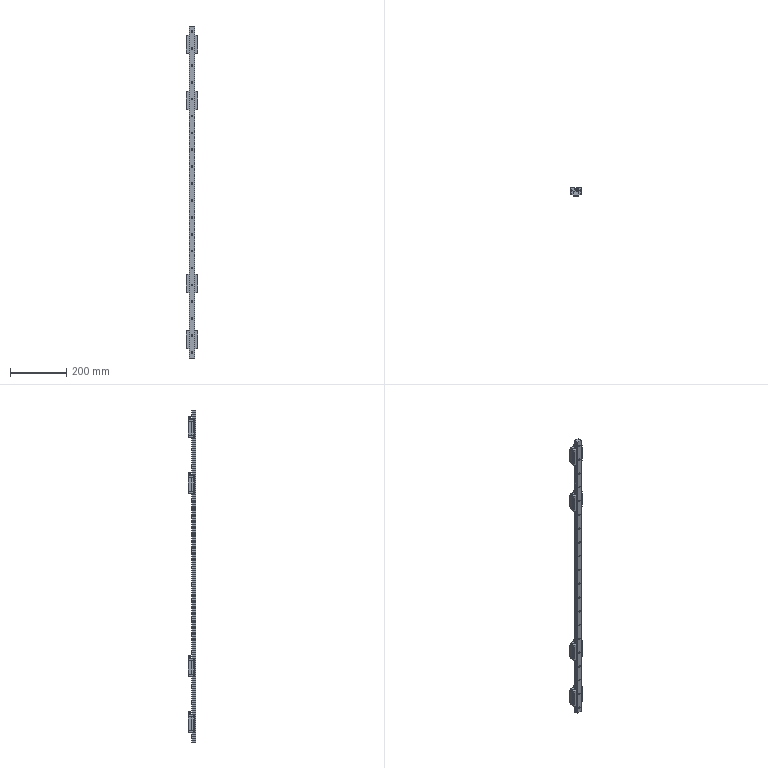Part | SolidWorks | 5 solids | 883 faces | box 42 x 28 x 1180 mm | volume 516437 mm3 | plane 454 | cylinder 317 | cone 108 | spline 4 | commonest cylinder face diameters 3.08 x80 6 x40 9.5 x40 4.134 x32 4.4 x32 4.8 x32